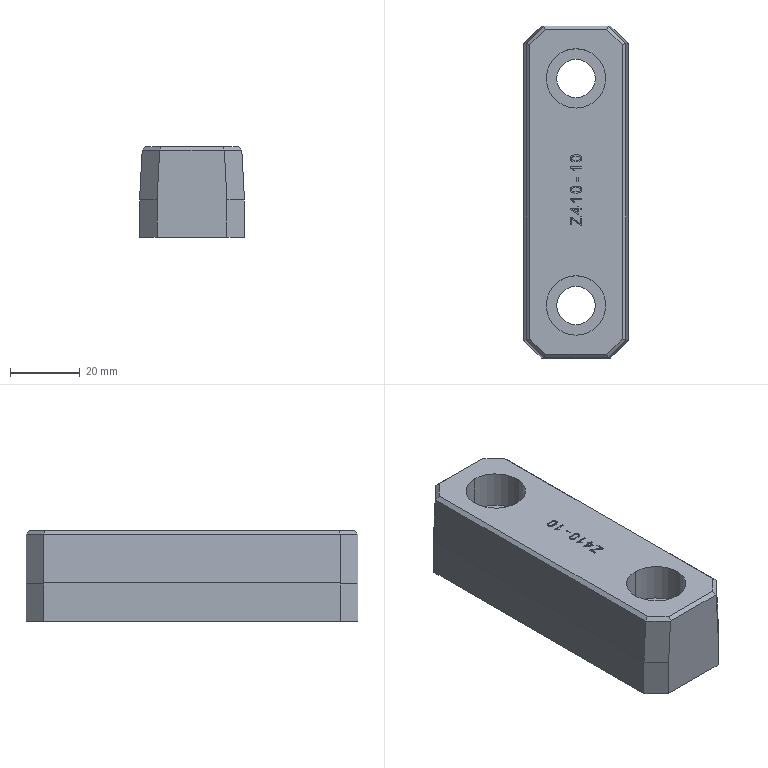Part | Creo | 1 solid | 132 faces | box 30 x 95 x 26 mm | volume 63715 mm3 | plane 70 | other 53 | cylinder 9 | commonest cylinder face diameters 11 x4 17 x4 45.582 x1